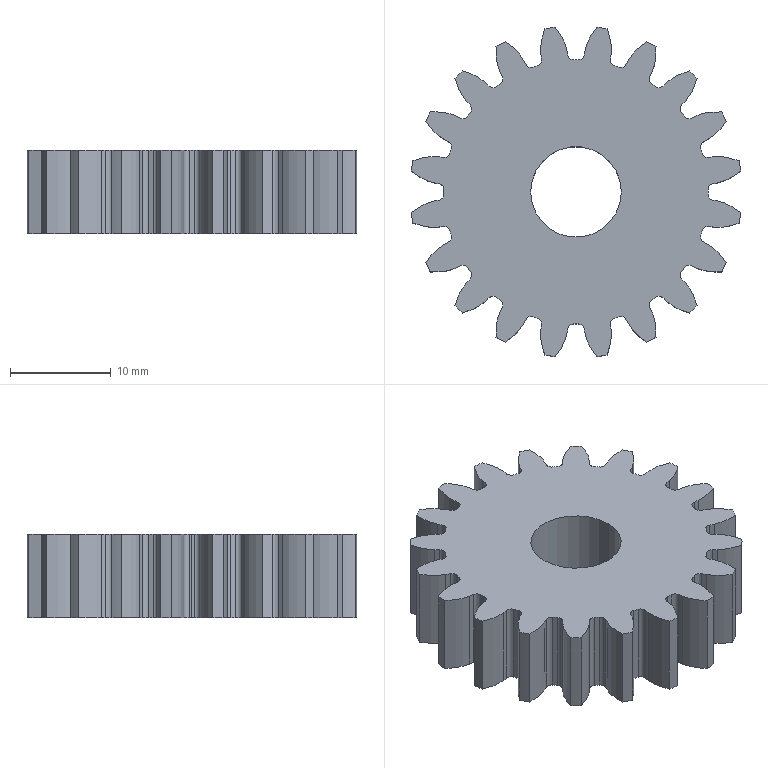Part | SolidWorks | features Extrusion 1 | 1 solid | 175 faces | box 32.74 x 32.74 x 8.27 mm | volume 5212 mm3 | cylinder 93 | plane 42 | spline 40 | commonest cylinder face diameters 1.14 x50 26.25 x21 33 x20 9 x2